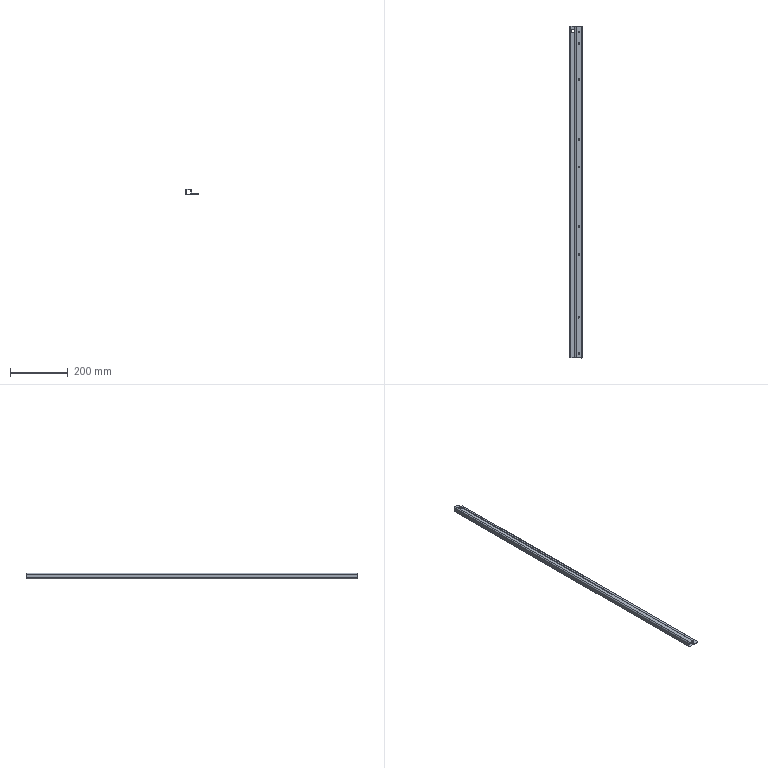Part | NX | features BREP 1 | 1 solid | 165 faces | box 42.999 x 1150 x 20.019 mm | volume 254430 mm3 | plane 111 | cylinder 36 | cone 18 | commonest cylinder face diameters 5.1 x18 4 x5 8 x5 4.1 x4 10 x4